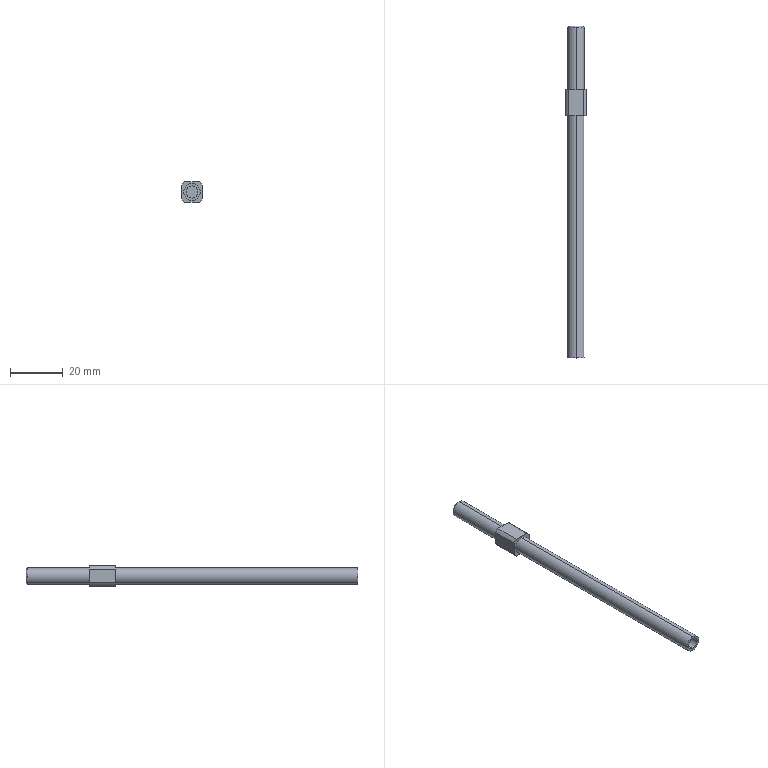Part | SolidWorks | features BaseBody 1 | 1 solid | 21 faces | box 7.938 x 125.5 x 7.703 mm | volume 2745 mm3 | cylinder 10 | plane 9 | cone 2 | commonest cylinder face diameters 6.35 x4 9.525 x4 4.564 x2
STEP:
#1=CARTESIAN_POINT('',(0.,-91.5,2.282));
#2=VERTEX_POINT('',#1);
#3=CARTESIAN_POINT('',(0.,-91.5,-2.282));
#4=VERTEX_POINT('',#3);
#5=CARTESIAN_POINT('',(0.,-91.5,0.));
#6=DIRECTION('',(0.,-1.,0.));
#7=DIRECTION('',(0.,0.,1.));
#8=AXIS2_PLACEMENT_3D('',#5,#6,#7);
#9=CIRCLE('',#8,2.282);
#10=EDGE_CURVE('',#2,#4,#9,.T.);
#11=ORIENTED_EDGE('',*,*,#10,.T.);
#12=CARTESIAN_POINT('',(0.,0.,-2.282));
#13=VERTEX_POINT('',#12);
#14=CARTESIAN_POINT('',(0.,-91.5,-2.282));
#15=DIRECTION('',(0.,1.,0.));
#16=VECTOR('',#15,1000.);
#17=LINE('',#14,#16);
#18=EDGE_CURVE('',#4,#13,#17,.T.);
#19=ORIENTED_EDGE('',*,*,#18,.T.);
#20=CARTESIAN_POINT('',(0.,0.,2.282));
#21=VERTEX_POINT('',#20);
#22=CARTESIAN_POINT('',(0.,0.,0.));
#23=DIRECTION('',(0.,1.,0.));
#24=DIRECTION('',(0.,0.,1.));
#25=AXIS2_PLACEMENT_3D('',#22,#23,#24);
#26=CIRCLE('',#25,2.282);
#27=EDGE_CURVE('',#13,#21,#26,.T.);
#28=ORIENTED_EDGE('',*,*,#27,.T.);
#29=CARTESIAN_POINT('',(0.,-91.5,2.282));
#30=DIRECTION('',(0.,1.,0.));
#31=VECTOR('',#30,1000.);
#32=LINE('',#29,#31);
#33=EDGE_CURVE('',#2,#21,#32,.T.);
#34=ORIENTED_EDGE('',*,*,#33,.F.);
#35=EDGE_LOOP('',(#11,#19,#28,#34));
#36=FACE_OUTER_BOUND('',#35,.T.);
#37=CARTESIAN_POINT('',(0.,-91.5,0.));
#38=DIRECTION('',(0.,1.,0.));
#39=DIRECTION('',(0.,0.,1.));
#40=AXIS2_PLACEMENT_3D('',#37,#38,#39);
#41=CYLINDRICAL_SURFACE('',#40,2.282);
#42=ADVANCED_FACE('',(#36),#41,.F.);
#43=CARTESIAN_POINT('',(0.,-91.5,3.175));
#44=VERTEX_POINT('',#43);
#45=CARTESIAN_POINT('',(0.,-91.5,-3.175));
#46=VERTEX_POINT('',#45);
#47=CARTESIAN_POINT('',(0.,-91.5,0.));
#48=DIRECTION('',(0.,1.,0.));
#49=DIRECTION('',(0.,0.,1.));
#50=AXIS2_PLACEMENT_3D('',#47,#48,#49);
#51=CIRCLE('',#50,3.175);
#52=EDGE_CURVE('',#44,#46,#51,.T.);
#53=ORIENTED_EDGE('',*,*,#52,.T.);
#54=CARTESIAN_POINT('',(0.,0.,-3.175));
#55=VERTEX_POINT('',#54);
#56=CARTESIAN_POINT('',(0.,-91.5,-3.175));
#57=DIRECTION('',(0.,1.,0.));
#58=VECTOR('',#57,1000.);
#59=LINE('',#56,#58);
#60=EDGE_CURVE('',#46,#55,#59,.T.);
#61=ORIENTED_EDGE('',*,*,#60,.T.);
#62=CARTESIAN_POINT('',(0.,0.,3.175));
#63=VERTEX_POINT('',#62);
#64=CARTESIAN_POINT('',(0.,0.,0.));
#65=DIRECTION('',(0.,1.,0.));
#66=DIRECTION('',(0.,0.,1.));
#67=AXIS2_PLACEMENT_3D('',#64,#65,#66);
#68=CIRCLE('',#67,3.175);
#69=EDGE_CURVE('',#63,#55,#68,.T.);
#70=ORIENTED_EDGE('',*,*,#69,.F.);
#71=CARTESIAN_POINT('',(0.,-91.5,3.175));
#72=DIRECTION('',(0.,1.,0.));
#73=VECTOR('',#72,1000.);
#74=LINE('',#71,#73);
#75=EDGE_CURVE('',#44,#63,#74,.T.);
#76=ORIENTED_EDGE('',*,*,#75,.F.);
#77=EDGE_LOOP('',(#53,#61,#70,#76));
#78=FACE_OUTER_BOUND('',#77,.T.);
#79=CARTESIAN_POINT('',(0.,-91.5,0.));
#80=DIRECTION('',(0.,1.,0.));
#81=DIRECTION('',(0.,0.,1.));
#82=AXIS2_PLACEMENT_3D('',#79,#80,#81);
#83=CYLINDRICAL_SURFACE('',#82,3.175);
#84=ADVANCED_FACE('',(#78),#83,.T.);
#85=CARTESIAN_POINT('',(0.,10.,3.175));
#86=VERTEX_POINT('',#85);
#87=CARTESIAN_POINT('',(0.,10.,-3.175));
#88=VERTEX_POINT('',#87);
#89=CARTESIAN_POINT('',(0.,10.,0.));
#90=DIRECTION('',(0.,1.,0.));
#91=DIRECTION('',(0.,0.,1.));
#92=AXIS2_PLACEMENT_3D('',#89,#90,#91);
#93=CIRCLE('',#92,3.175);
#94=EDGE_CURVE('',#86,#88,#93,.T.);
#95=ORIENTED_EDGE('',*,*,#94,.T.);
#96=CARTESIAN_POINT('',(0.,33.492,-3.175));
#97=VERTEX_POINT('',#96);
#98=CARTESIAN_POINT('',(0.,10.,-3.175));
#99=DIRECTION('',(0.,1.,0.));
#100=VECTOR('',#99,1000.);
#101=LINE('',#98,#100);
#102=EDGE_CURVE('',#88,#97,#101,.T.);
#103=ORIENTED_EDGE('',*,*,#102,.T.);
#104=CARTESIAN_POINT('',(0.,33.492,3.175));
#105=VERTEX_POINT('',#104);
#106=CARTESIAN_POINT('',(0.,33.492,0.));
#107=DIRECTION('',(0.,1.,0.));
#108=DIRECTION('',(-1.,0.,0.));
#109=AXIS2_PLACEMENT_3D('',#106,#107,#108);
#110=CIRCLE('',#109,3.175);
#111=EDGE_CURVE('',#105,#97,#110,.T.);
#112=ORIENTED_EDGE('',*,*,#111,.F.);
#113=CARTESIAN_POINT('',(0.,10.,3.175));
#114=DIRECTION('',(0.,1.,0.));
#115=VECTOR('',#114,1000.);
#116=LINE('',#113,#115);
#117=EDGE_CURVE('',#86,#105,#116,.T.);
#118=ORIENTED_EDGE('',*,*,#117,.F.);
#119=EDGE_LOOP('',(#95,#103,#112,#118));
#120=FACE_OUTER_BOUND('',#119,.T.);
#121=CARTESIAN_POINT('',(0.,10.,0.));
#122=DIRECTION('',(0.,1.,0.));
#123=DIRECTION('',(0.,0.,1.));
#124=AXIS2_PLACEMENT_3D('',#121,#122,#123);
#125=CYLINDRICAL_SURFACE('',#124,3.175);
#126=ADVANCED_FACE('',(#120),#125,.T.);
#127=CARTESIAN_POINT('',(0.,34.,2.667));
#128=VERTEX_POINT('',#127);
#129=CARTESIAN_POINT('',(0.,34.,-2.667));
#130=VERTEX_POINT('',#129);
#131=CARTESIAN_POINT('',(0.,34.,0.));
#132=DIRECTION('',(0.,1.,0.));
#133=DIRECTION('',(0.,0.,-1.));
#134=AXIS2_PLACEMENT_3D('',#131,#132,#133);
#135=CIRCLE('',#134,2.667);
#136=EDGE_CURVE('',#128,#130,#135,.T.);
#137=ORIENTED_EDGE('',*,*,#136,.F.);
#138=CARTESIAN_POINT('',(0.,34.,2.667));
#139=DIRECTION('',(0.,-0.7071,0.7071));
#140=VECTOR('',#139,1000.);
#141=LINE('',#138,#140);
#142=EDGE_CURVE('',#128,#105,#141,.T.);
#143=ORIENTED_EDGE('',*,*,#142,.T.);
#144=ORIENTED_EDGE('',*,*,#111,.T.);
#145=CARTESIAN_POINT('',(0.,34.,-2.667));
#146=DIRECTION('',(0.,-0.7071,-0.7071));
#147=VECTOR('',#146,1000.);
#148=LINE('',#145,#147);
#149=EDGE_CURVE('',#130,#97,#148,.T.);
#150=ORIENTED_EDGE('',*,*,#149,.F.);
#151=EDGE_LOOP('',(#137,#143,#144,#150));
#152=FACE_OUTER_BOUND('',#151,.T.);
#153=CARTESIAN_POINT('',(0.,34.,0.));
#154=DIRECTION('',(0.,-1.,0.));
#155=DIRECTION('',(0.,0.,-1.));
#156=AXIS2_PLACEMENT_3D('',#153,#154,#155);
#157=CONICAL_SURFACE('',#156,2.667,0.7854);
#158=ADVANCED_FACE('',(#152),#157,.T.);
#159=ORIENTED_EDGE('',*,*,#18,.F.);
#160=CARTESIAN_POINT('',(0.,-91.5,0.));
#161=DIRECTION('',(0.,-1.,0.));
#162=DIRECTION('',(0.,0.,1.));
#163=AXIS2_PLACEMENT_3D('',#160,#161,#162);
#164=CIRCLE('',#163,2.282);
#165=EDGE_CURVE('',#4,#2,#164,.T.);
#166=ORIENTED_EDGE('',*,*,#165,.T.);
#167=ORIENTED_EDGE('',*,*,#33,.T.);
#168=CARTESIAN_POINT('',(0.,0.,0.));
#169=DIRECTION('',(0.,1.,0.));
#170=DIRECTION('',(0.,0.,1.));
#171=AXIS2_PLACEMENT_3D('',#168,#169,#170);
#172=CIRCLE('',#171,2.282);
#173=EDGE_CURVE('',#21,#13,#172,.T.);
#174=ORIENTED_EDGE('',*,*,#173,.T.);
#175=EDGE_LOOP('',(#159,#166,#167,#174));
#176=FACE_OUTER_BOUND('',#175,.T.);
#177=CARTESIAN_POINT('',(0.,-91.5,0.));
#178=DIRECTION('',(0.,1.,0.));
#179=DIRECTION('',(0.,0.,1.));
#180=AXIS2_PLACEMENT_3D('',#177,#178,#179);
#181=CYLINDRICAL_SURFACE('',#180,2.282);
#182=ADVANCED_FACE('',(#176),#181,.F.);
#183=ORIENTED_EDGE('',*,*,#173,.F.);
#184=ORIENTED_EDGE('',*,*,#27,.F.);
#185=EDGE_LOOP('',(#183,#184));
#186=FACE_OUTER_BOUND('',#185,.T.);
#187=CARTESIAN_POINT('',(2.309,0.,-2.309));
#188=DIRECTION('',(0.,1.,0.));
#189=DIRECTION('',(-1.,0.,0.));
#190=AXIS2_PLACEMENT_3D('',#187,#188,#189);
#191=PLANE('',#190);
#192=ADVANCED_FACE('',(#186),#191,.F.);
#193=ORIENTED_EDGE('',*,*,#10,.F.);
#194=ORIENTED_EDGE('',*,*,#165,.F.);
#195=EDGE_LOOP('',(#193,#194));
#196=FACE_BOUND('',#195,.T.);
#197=ORIENTED_EDGE('',*,*,#52,.F.);
#198=CARTESIAN_POINT('',(0.,-91.5,0.));
#199=DIRECTION('',(0.,1.,0.));
#200=DIRECTION('',(0.,0.,1.));
#201=AXIS2_PLACEMENT_3D('',#198,#199,#200);
#202=CIRCLE('',#201,3.175);
#203=EDGE_CURVE('',#46,#44,#202,.T.);
#204=ORIENTED_EDGE('',*,*,#203,.F.);
#205=EDGE_LOOP('',(#197,#204));
#206=FACE_OUTER_BOUND('',#205,.T.);
#207=CARTESIAN_POINT('',(3.213,-91.5,-3.213));
#208=DIRECTION('',(0.,1.,0.));
#209=DIRECTION('',(-1.,0.,0.));
#210=AXIS2_PLACEMENT_3D('',#207,#208,#209);
#211=PLANE('',#210);
#212=ADVANCED_FACE('',(#196,#206),#211,.F.);
#213=ORIENTED_EDGE('',*,*,#60,.F.);
#214=ORIENTED_EDGE('',*,*,#203,.T.);
#215=ORIENTED_EDGE('',*,*,#75,.T.);
#216=CARTESIAN_POINT('',(0.,0.,0.));
#217=DIRECTION('',(0.,1.,0.));
#218=DIRECTION('',(0.,0.,1.));
#219=AXIS2_PLACEMENT_3D('',#216,#217,#218);
#220=CIRCLE('',#219,3.175);
#221=EDGE_CURVE('',#55,#63,#220,.T.);
#222=ORIENTED_EDGE('',*,*,#221,.F.);
#223=EDGE_LOOP('',(#213,#214,#215,#222));
#224=FACE_OUTER_BOUND('',#223,.T.);
#225=CARTESIAN_POINT('',(0.,-91.5,0.));
#226=DIRECTION('',(0.,1.,0.));
#227=DIRECTION('',(0.,0.,1.));
#228=AXIS2_PLACEMENT_3D('',#225,#226,#227);
#229=CYLINDRICAL_SURFACE('',#228,3.175);
#230=ADVANCED_FACE('',(#224),#229,.T.);
#231=ORIENTED_EDGE('',*,*,#69,.T.);
#232=ORIENTED_EDGE('',*,*,#221,.T.);
#233=EDGE_LOOP('',(#231,#232));
#234=FACE_BOUND('',#233,.T.);
#235=CARTESIAN_POINT('',(-3.969,0.,-2.633));
#236=VERTEX_POINT('',#235);
#237=CARTESIAN_POINT('',(-2.801,0.,-3.852));
#238=VERTEX_POINT('',#237);
#239=CARTESIAN_POINT('',(0.,0.,0.));
#240=DIRECTION('',(0.,-1.,0.));
#241=DIRECTION('',(0.,0.,1.));
#242=AXIS2_PLACEMENT_3D('',#239,#240,#241);
#243=CIRCLE('',#242,4.762);
#244=EDGE_CURVE('',#236,#238,#243,.T.);
#245=ORIENTED_EDGE('',*,*,#244,.T.);
#246=CARTESIAN_POINT('',(2.801,0.,-3.852));
#247=VERTEX_POINT('',#246);
#248=CARTESIAN_POINT('',(0.,0.,-3.852));
#249=DIRECTION('',(-1.,0.,0.));
#250=VECTOR('',#249,1000.);
#251=LINE('',#248,#250);
#252=EDGE_CURVE('',#247,#238,#251,.T.);
#253=ORIENTED_EDGE('',*,*,#252,.F.);
#254=CARTESIAN_POINT('',(3.969,0.,-2.633));
#255=VERTEX_POINT('',#254);
#256=CARTESIAN_POINT('',(0.,0.,0.));
#257=DIRECTION('',(0.,-1.,0.));
#258=DIRECTION('',(0.,0.,1.));
#259=AXIS2_PLACEMENT_3D('',#256,#257,#258);
#260=CIRCLE('',#259,4.762);
#261=EDGE_CURVE('',#247,#255,#260,.T.);
#262=ORIENTED_EDGE('',*,*,#261,.T.);
#263=CARTESIAN_POINT('',(3.969,0.,2.633));
#264=VERTEX_POINT('',#263);
#265=CARTESIAN_POINT('',(3.969,0.,0.));
#266=DIRECTION('',(0.,0.,-1.));
#267=VECTOR('',#266,1000.);
#268=LINE('',#265,#267);
#269=EDGE_CURVE('',#264,#255,#268,.T.);
#270=ORIENTED_EDGE('',*,*,#269,.F.);
#271=CARTESIAN_POINT('',(2.801,0.,3.852));
#272=VERTEX_POINT('',#271);
#273=CARTESIAN_POINT('',(0.,0.,0.));
#274=DIRECTION('',(0.,-1.,0.));
#275=DIRECTION('',(0.,0.,1.));
#276=AXIS2_PLACEMENT_3D('',#273,#274,#275);
#277=CIRCLE('',#276,4.762);
#278=EDGE_CURVE('',#264,#272,#277,.T.);
#279=ORIENTED_EDGE('',*,*,#278,.T.);
#280=CARTESIAN_POINT('',(-2.801,0.,3.852));
#281=VERTEX_POINT('',#280);
#282=CARTESIAN_POINT('',(0.,0.,3.852));
#283=DIRECTION('',(1.,0.,0.));
#284=VECTOR('',#283,1000.);
#285=LINE('',#282,#284);
#286=EDGE_CURVE('',#281,#272,#285,.T.);
#287=ORIENTED_EDGE('',*,*,#286,.F.);
#288=CARTESIAN_POINT('',(-3.969,0.,2.633));
#289=VERTEX_POINT('',#288);
#290=CARTESIAN_POINT('',(0.,0.,0.));
#291=DIRECTION('',(0.,-1.,0.));
#292=DIRECTION('',(0.,0.,1.));
#293=AXIS2_PLACEMENT_3D('',#290,#291,#292);
#294=CIRCLE('',#293,4.762);
#295=EDGE_CURVE('',#281,#289,#294,.T.);
#296=ORIENTED_EDGE('',*,*,#295,.T.);
#297=CARTESIAN_POINT('',(-3.969,0.,0.));
#298=DIRECTION('',(0.,0.,1.));
#299=VECTOR('',#298,1000.);
#300=LINE('',#297,#299);
#301=EDGE_CURVE('',#236,#289,#300,.T.);
#302=ORIENTED_EDGE('',*,*,#301,.F.);
#303=EDGE_LOOP('',(#245,#253,#262,#270,#279,#287,#296,#302));
#304=FACE_OUTER_BOUND('',#303,.T.);
#305=CARTESIAN_POINT('',(3.969,0.,-3.852));
#306=DIRECTION('',(0.,1.,0.));
#307=DIRECTION('',(-1.,0.,0.));
#308=AXIS2_PLACEMENT_3D('',#305,#306,#307);
#309=PLANE('',#308);
#310=ADVANCED_FACE('',(#234,#304),#309,.F.);
#311=ORIENTED_EDGE('',*,*,#301,.T.);
#312=CARTESIAN_POINT('',(-3.969,10.,2.633));
#313=VERTEX_POINT('',#312);
#314=CARTESIAN_POINT('',(-3.969,5.,2.633));
#315=DIRECTION('',(0.,1.,0.));
#316=VECTOR('',#315,1000.);
#317=LINE('',#314,#316);
#318=EDGE_CURVE('',#289,#313,#317,.T.);
#319=ORIENTED_EDGE('',*,*,#318,.T.);
#320=CARTESIAN_POINT('',(-3.969,10.,-2.633));
#321=VERTEX_POINT('',#320);
#322=CARTESIAN_POINT('',(-3.969,10.,0.));
#323=DIRECTION('',(0.,0.,-1.));
#324=VECTOR('',#323,1000.);
#325=LINE('',#322,#324);
#326=EDGE_CURVE('',#313,#321,#325,.T.);
#327=ORIENTED_EDGE('',*,*,#326,.T.);
#328=CARTESIAN_POINT('',(-3.969,5.,-2.633));
#329=DIRECTION('',(0.,-1.,0.));
#330=VECTOR('',#329,1000.);
#331=LINE('',#328,#330);
#332=EDGE_CURVE('',#321,#236,#331,.T.);
#333=ORIENTED_EDGE('',*,*,#332,.T.);
#334=EDGE_LOOP('',(#311,#319,#327,#333));
#335=FACE_OUTER_BOUND('',#334,.T.);
#336=CARTESIAN_POINT('',(-3.969,0.,-2.633));
#337=DIRECTION('',(-1.,0.,0.));
#338=DIRECTION('',(0.,0.,1.));
#339=AXIS2_PLACEMENT_3D('',#336,#337,#338);
#340=PLANE('',#339);
#341=ADVANCED_FACE('',(#335),#340,.T.);
#342=ORIENTED_EDGE('',*,*,#252,.T.);
#343=CARTESIAN_POINT('',(-2.801,10.,-3.852));
#344=VERTEX_POINT('',#343);
#345=CARTESIAN_POINT('',(-2.801,5.,-3.852));
#346=DIRECTION('',(0.,1.,0.));
#347=VECTOR('',#346,1000.);
#348=LINE('',#345,#347);
#349=EDGE_CURVE('',#238,#344,#348,.T.);
#350=ORIENTED_EDGE('',*,*,#349,.T.);
#351=CARTESIAN_POINT('',(2.801,10.,-3.852));
#352=VERTEX_POINT('',#351);
#353=CARTESIAN_POINT('',(0.,10.,-3.852));
#354=DIRECTION('',(1.,0.,0.));
#355=VECTOR('',#354,1000.);
#356=LINE('',#353,#355);
#357=EDGE_CURVE('',#344,#352,#356,.T.);
#358=ORIENTED_EDGE('',*,*,#357,.T.);
#359=CARTESIAN_POINT('',(2.801,5.,-3.852));
#360=DIRECTION('',(0.,-1.,0.));
#361=VECTOR('',#360,1000.);
#362=LINE('',#359,#361);
#363=EDGE_CURVE('',#352,#247,#362,.T.);
#364=ORIENTED_EDGE('',*,*,#363,.T.);
#365=EDGE_LOOP('',(#342,#350,#358,#364));
#366=FACE_OUTER_BOUND('',#365,.T.);
#367=CARTESIAN_POINT('',(2.801,0.,-3.852));
#368=DIRECTION('',(0.,0.,-1.));
#369=DIRECTION('',(-1.,0.,0.));
#370=AXIS2_PLACEMENT_3D('',#367,#368,#369);
#371=PLANE('',#370);
#372=ADVANCED_FACE('',(#366),#371,.T.);
#373=ORIENTED_EDGE('',*,*,#269,.T.);
#374=CARTESIAN_POINT('',(3.969,10.,-2.633));
#375=VERTEX_POINT('',#374);
#376=CARTESIAN_POINT('',(3.969,5.,-2.633));
#377=DIRECTION('',(0.,1.,0.));
#378=VECTOR('',#377,1000.);
#379=LINE('',#376,#378);
#380=EDGE_CURVE('',#255,#375,#379,.T.);
#381=ORIENTED_EDGE('',*,*,#380,.T.);
#382=CARTESIAN_POINT('',(3.969,10.,2.633));
#383=VERTEX_POINT('',#382);
#384=CARTESIAN_POINT('',(3.969,10.,0.));
#385=DIRECTION('',(0.,0.,1.));
#386=VECTOR('',#385,1000.);
#387=LINE('',#384,#386);
#388=EDGE_CURVE('',#375,#383,#387,.T.);
#389=ORIENTED_EDGE('',*,*,#388,.T.);
#390=CARTESIAN_POINT('',(3.969,5.,2.633));
#391=DIRECTION('',(0.,-1.,0.));
#392=VECTOR('',#391,1000.);
#393=LINE('',#390,#392);
#394=EDGE_CURVE('',#383,#264,#393,.T.);
#395=ORIENTED_EDGE('',*,*,#394,.T.);
#396=EDGE_LOOP('',(#373,#381,#389,#395));
#397=FACE_OUTER_BOUND('',#396,.T.);
#398=CARTESIAN_POINT('',(3.969,0.,-2.633));
#399=DIRECTION('',(1.,0.,0.));
#400=DIRECTION('',(0.,1.,0.));
#401=AXIS2_PLACEMENT_3D('',#398,#399,#400);
#402=PLANE('',#401);
#403=ADVANCED_FACE('',(#397),#402,.T.);
#404=ORIENTED_EDGE('',*,*,#286,.T.);
#405=CARTESIAN_POINT('',(2.801,10.,3.852));
#406=VERTEX_POINT('',#405);
#407=CARTESIAN_POINT('',(2.801,5.,3.852));
#408=DIRECTION('',(0.,1.,0.));
#409=VECTOR('',#408,1000.);
#410=LINE('',#407,#409);
#411=EDGE_CURVE('',#272,#406,#410,.T.);
#412=ORIENTED_EDGE('',*,*,#411,.T.);
#413=CARTESIAN_POINT('',(-2.801,10.,3.852));
#414=VERTEX_POINT('',#413);
#415=CARTESIAN_POINT('',(0.,10.,3.852));
#416=DIRECTION('',(-1.,0.,0.));
#417=VECTOR('',#416,1000.);
#418=LINE('',#415,#417);
#419=EDGE_CURVE('',#406,#414,#418,.T.);
#420=ORIENTED_EDGE('',*,*,#419,.T.);
#421=CARTESIAN_POINT('',(-2.801,5.,3.852));
#422=DIRECTION('',(0.,-1.,0.));
#423=VECTOR('',#422,1000.);
#424=LINE('',#421,#423);
#425=EDGE_CURVE('',#414,#281,#424,.T.);
#426=ORIENTED_EDGE('',*,*,#425,.T.);
#427=EDGE_LOOP('',(#404,#412,#420,#426));
#428=FACE_OUTER_BOUND('',#427,.T.);
#429=CARTESIAN_POINT('',(-2.801,0.,3.852));
#430=DIRECTION('',(0.,0.,1.));
#431=DIRECTION('',(1.,0.,0.));
#432=AXIS2_PLACEMENT_3D('',#429,#430,#431);
#433=PLANE('',#432);
#434=ADVANCED_FACE('',(#428),#433,.T.);
#435=ORIENTED_EDGE('',*,*,#295,.F.);
#436=ORIENTED_EDGE('',*,*,#425,.F.);
#437=CARTESIAN_POINT('',(0.,10.,0.));
#438=DIRECTION('',(0.,1.,0.));
#439=DIRECTION('',(0.,0.,1.));
#440=AXIS2_PLACEMENT_3D('',#437,#438,#439);
#441=CIRCLE('',#440,4.762);
#442=EDGE_CURVE('',#313,#414,#441,.T.);
#443=ORIENTED_EDGE('',*,*,#442,.F.);
#444=ORIENTED_EDGE('',*,*,#318,.F.);
#445=EDGE_LOOP('',(#435,#436,#443,#444));
#446=FACE_OUTER_BOUND('',#445,.T.);
#447=CARTESIAN_POINT('',(0.,0.,0.));
#448=DIRECTION('',(0.,1.,0.));
#449=DIRECTION('',(0.,0.,1.));
#450=AXIS2_PLACEMENT_3D('',#447,#448,#449);
#451=CYLINDRICAL_SURFACE('',#450,4.762);
#452=ADVANCED_FACE('',(#446),#451,.T.);
#453=CARTESIAN_POINT('',(0.,10.,0.));
#454=DIRECTION('',(0.,1.,0.));
#455=DIRECTION('',(0.,0.,1.));
#456=AXIS2_PLACEMENT_3D('',#453,#454,#455);
#457=CIRCLE('',#456,4.762);
#458=EDGE_CURVE('',#344,#321,#457,.T.);
#459=ORIENTED_EDGE('',*,*,#458,.F.);
#460=ORIENTED_EDGE('',*,*,#349,.F.);
#461=ORIENTED_EDGE('',*,*,#244,.F.);
#462=ORIENTED_EDGE('',*,*,#332,.F.);
#463=EDGE_LOOP('',(#459,#460,#461,#462));
#464=FACE_OUTER_BOUND('',#463,.T.);
#465=CARTESIAN_POINT('',(0.,0.,0.));
#466=DIRECTION('',(0.,1.,0.));
#467=DIRECTION('',(0.,0.,1.));
#468=AXIS2_PLACEMENT_3D('',#465,#466,#467);
#469=CYLINDRICAL_SURFACE('',#468,4.762);
#470=ADVANCED_FACE('',(#464),#469,.T.);
#471=ORIENTED_EDGE('',*,*,#94,.F.);
#472=CARTESIAN_POINT('',(0.,10.,0.));
#473=DIRECTION('',(0.,1.,0.));
#474=DIRECTION('',(0.,0.,1.));
#475=AXIS2_PLACEMENT_3D('',#472,#473,#474);
#476=CIRCLE('',#475,3.175);
#477=EDGE_CURVE('',#88,#86,#476,.T.);
#478=ORIENTED_EDGE('',*,*,#477,.F.);
#479=EDGE_LOOP('',(#471,#478));
#480=FACE_BOUND('',#479,.T.);
#481=ORIENTED_EDGE('',*,*,#442,.T.);
#482=ORIENTED_EDGE('',*,*,#419,.F.);
#483=CARTESIAN_POINT('',(0.,10.,0.));
#484=DIRECTION('',(0.,-1.,0.));
#485=DIRECTION('',(0.,0.,1.));
#486=AXIS2_PLACEMENT_3D('',#483,#484,#485);
#487=CIRCLE('',#486,4.762);
#488=EDGE_CURVE('',#383,#406,#487,.T.);
#489=ORIENTED_EDGE('',*,*,#488,.F.);
#490=ORIENTED_EDGE('',*,*,#388,.F.);
#491=CARTESIAN_POINT('',(0.,10.,0.));
#492=DIRECTION('',(0.,-1.,0.));
#493=DIRECTION('',(0.,0.,1.));
#494=AXIS2_PLACEMENT_3D('',#491,#492,#493);
#495=CIRCLE('',#494,4.762);
#496=EDGE_CURVE('',#352,#375,#495,.T.);
#497=ORIENTED_EDGE('',*,*,#496,.F.);
#498=ORIENTED_EDGE('',*,*,#357,.F.);
#499=ORIENTED_EDGE('',*,*,#458,.T.);
#500=ORIENTED_EDGE('',*,*,#326,.F.);
#501=EDGE_LOOP('',(#481,#482,#489,#490,#497,#498,#499,#500));
#502=FACE_OUTER_BOUND('',#501,.T.);
#503=CARTESIAN_POINT('',(-3.969,10.,-3.852));
#504=DIRECTION('',(0.,-1.,0.));
#505=DIRECTION('',(1.,0.,0.));
#506=AXIS2_PLACEMENT_3D('',#503,#504,#505);
#507=PLANE('',#506);
#508=ADVANCED_FACE('',(#480,#502),#507,.F.);
#509=ORIENTED_EDGE('',*,*,#496,.T.);
#510=ORIENTED_EDGE('',*,*,#380,.F.);
#511=ORIENTED_EDGE('',*,*,#261,.F.);
#512=ORIENTED_EDGE('',*,*,#363,.F.);
#513=EDGE_LOOP('',(#509,#510,#511,#512));
#514=FACE_OUTER_BOUND('',#513,.T.);
#515=CARTESIAN_POINT('',(0.,0.,0.));
#516=DIRECTION('',(0.,1.,0.));
#517=DIRECTION('',(0.,0.,1.));
#518=AXIS2_PLACEMENT_3D('',#515,#516,#517);
#519=CYLINDRICAL_SURFACE('',#518,4.762);
#520=ADVANCED_FACE('',(#514),#519,.T.);
#521=ORIENTED_EDGE('',*,*,#488,.T.);
#522=ORIENTED_EDGE('',*,*,#411,.F.);
#523=ORIENTED_EDGE('',*,*,#278,.F.);
#524=ORIENTED_EDGE('',*,*,#394,.F.);
#525=EDGE_LOOP('',(#521,#522,#523,#524));
#526=FACE_OUTER_BOUND('',#525,.T.);
#527=CARTESIAN_POINT('',(0.,0.,0.));
#528=DIRECTION('',(0.,1.,0.));
#529=DIRECTION('',(0.,0.,1.));
#530=AXIS2_PLACEMENT_3D('',#527,#528,#529);
#531=CYLINDRICAL_SURFACE('',#530,4.762);
#532=ADVANCED_FACE('',(#526),#531,.T.);
#533=ORIENTED_EDGE('',*,*,#102,.F.);
#534=ORIENTED_EDGE('',*,*,#477,.T.);
#535=ORIENTED_EDGE('',*,*,#117,.T.);
#536=CARTESIAN_POINT('',(0.,33.492,0.));
#537=DIRECTION('',(0.,1.,0.));
#538=DIRECTION('',(-1.,0.,0.));
#539=AXIS2_PLACEMENT_3D('',#536,#537,#538);
#540=CIRCLE('',#539,3.175);
#541=EDGE_CURVE('',#97,#105,#540,.T.);
#542=ORIENTED_EDGE('',*,*,#541,.F.);
#543=EDGE_LOOP('',(#533,#534,#535,#542));
#544=FACE_OUTER_BOUND('',#543,.T.);
#545=CARTESIAN_POINT('',(0.,10.,0.));
#546=DIRECTION('',(0.,1.,0.));
#547=DIRECTION('',(0.,0.,1.));
#548=AXIS2_PLACEMENT_3D('',#545,#546,#547);
#549=CYLINDRICAL_SURFACE('',#548,3.175);
#550=ADVANCED_FACE('',(#544),#549,.T.);
#551=ORIENTED_EDGE('',*,*,#142,.F.);
#552=CARTESIAN_POINT('',(0.,34.,0.));
#553=DIRECTION('',(0.,1.,0.));
#554=DIRECTION('',(0.,0.,-1.));
#555=AXIS2_PLACEMENT_3D('',#552,#553,#554);
#556=CIRCLE('',#555,2.667);
#557=EDGE_CURVE('',#130,#128,#556,.T.);
#558=ORIENTED_EDGE('',*,*,#557,.F.);
#559=ORIENTED_EDGE('',*,*,#149,.T.);
#560=ORIENTED_EDGE('',*,*,#541,.T.);
#561=EDGE_LOOP('',(#551,#558,#559,#560));
#562=FACE_OUTER_BOUND('',#561,.T.);
#563=CARTESIAN_POINT('',(0.,34.,0.));
#564=DIRECTION('',(0.,-1.,0.));
#565=DIRECTION('',(0.,0.,-1.));
#566=AXIS2_PLACEMENT_3D('',#563,#564,#565);
#567=CONICAL_SURFACE('',#566,2.667,0.7854);
#568=ADVANCED_FACE('',(#562),#567,.T.);
#569=ORIENTED_EDGE('',*,*,#557,.T.);
#570=ORIENTED_EDGE('',*,*,#136,.T.);
#571=EDGE_LOOP('',(#569,#570));
#572=FACE_OUTER_BOUND('',#571,.T.);
#573=CARTESIAN_POINT('',(-2.699,34.,-2.699));
#574=DIRECTION('',(0.,-1.,0.));
#575=DIRECTION('',(1.,0.,0.));
#576=AXIS2_PLACEMENT_3D('',#573,#574,#575);
#577=PLANE('',#576);
#578=ADVANCED_FACE('',(#572),#577,.F.);
#579=CLOSED_SHELL('',(#42,#84,#126,#158,#182,#192,#212,#230,#310,#341,#372,#403,#434,#452,#470,#508,#520,#532,#550,#568,#578));
#580=MANIFOLD_SOLID_BREP('',#579);
#581=CARTESIAN_POINT('',(0.,0.,0.));
#582=DIRECTION('',(0.,0.,1.));
#583=DIRECTION('',(1.,0.,0.));
#584=AXIS2_PLACEMENT_3D('',#581,#582,#583);
#585=(LENGTH_UNIT()NAMED_UNIT(*)SI_UNIT(.MILLI.,.METRE.));
#586=UNCERTAINTY_MEASURE_WITH_UNIT(LENGTH_MEASURE(0.00001),#585,'','');
#587=(NAMED_UNIT(*)PLANE_ANGLE_UNIT()SI_UNIT($,.RADIAN.));
#588=(NAMED_UNIT(*)SI_UNIT($,.STERADIAN.)SOLID_ANGLE_UNIT());
#589=(GEOMETRIC_REPRESENTATION_CONTEXT(3)GLOBAL_UNCERTAINTY_ASSIGNED_CONTEXT((#586))GLOBAL_UNIT_ASSIGNED_CONTEXT((#585,#587,#588))REPRESENTATION_CONTEXT('',''));
#590=ADVANCED_BREP_SHAPE_REPRESENTATION('',(#580,#584),#589);